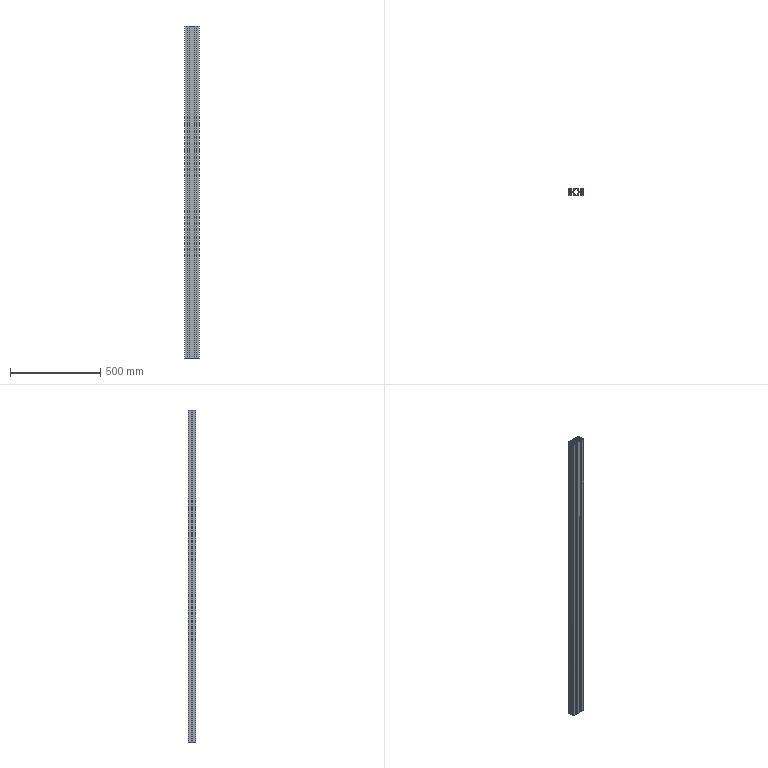Part | NX | 1 solid | 88 faces | box 80 x 40 x 1840 mm | volume 2229117 mm3 | plane 78 | cylinder 10 | commonest cylinder face diameters 6 x4 8 x4 6.75 x2